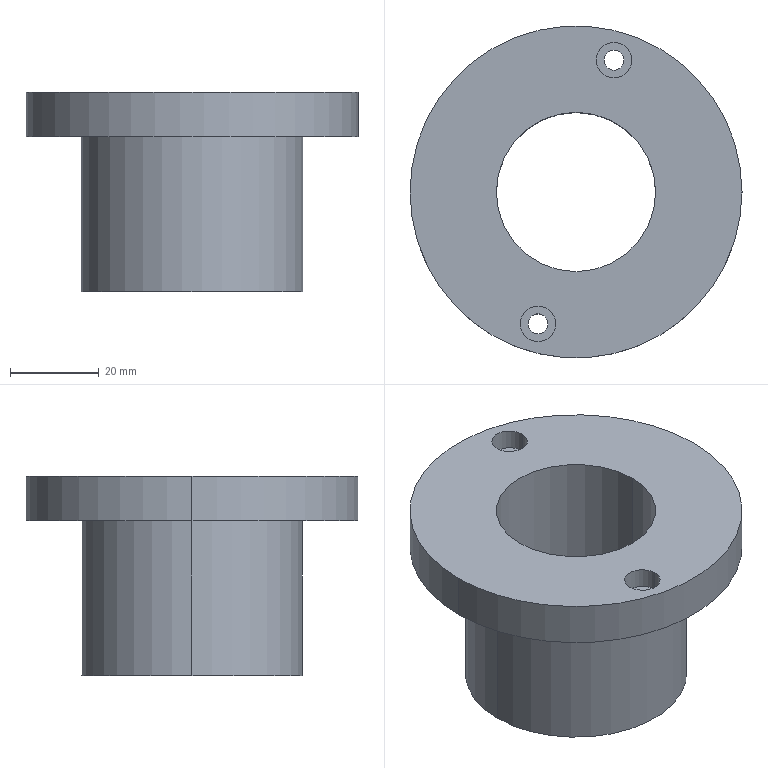Part | SolidWorks | features Extrusion 1, HoleWzd 1, ICE 1 | 1 solid | 19 faces | box 75 x 75 x 45 mm | volume 66462 mm3 | cylinder 14 | plane 5 | commonest cylinder face diameters 4.5 x4 8 x4 36 x2 50 x2 75 x2
STEP:
#1=CARTESIAN_POINT('',(-12.588,-29.787,40.4));
#2=VERTEX_POINT('',#1);
#3=CARTESIAN_POINT('',(-4.588,-29.787,40.4));
#4=VERTEX_POINT('',#3);
#5=CARTESIAN_POINT('',(-8.588,-29.787,40.4));
#6=DIRECTION('',(0.,0.,1.));
#7=DIRECTION('',(1.,0.,0.));
#8=AXIS2_PLACEMENT_3D('',#5,#6,#7);
#9=CIRCLE('',#8,4.);
#10=EDGE_CURVE('',#2,#4,#9,.T.);
#11=ORIENTED_EDGE('',*,*,#10,.F.);
#12=CARTESIAN_POINT('',(-12.588,-29.787,45.));
#13=VERTEX_POINT('',#12);
#14=CARTESIAN_POINT('',(-12.588,-29.787,45.));
#15=DIRECTION('',(0.,0.,1.));
#16=VECTOR('',#15,1000.);
#17=LINE('',#14,#16);
#18=EDGE_CURVE('',#2,#13,#17,.T.);
#19=ORIENTED_EDGE('',*,*,#18,.T.);
#20=CARTESIAN_POINT('',(-4.588,-29.787,45.));
#21=VERTEX_POINT('',#20);
#22=CARTESIAN_POINT('',(-8.588,-29.787,45.));
#23=DIRECTION('',(0.,0.,1.));
#24=DIRECTION('',(1.,0.,0.));
#25=AXIS2_PLACEMENT_3D('',#22,#23,#24);
#26=CIRCLE('',#25,4.);
#27=EDGE_CURVE('',#13,#21,#26,.T.);
#28=ORIENTED_EDGE('',*,*,#27,.T.);
#29=CARTESIAN_POINT('',(-4.588,-29.787,45.));
#30=DIRECTION('',(0.,0.,1.));
#31=VECTOR('',#30,1000.);
#32=LINE('',#29,#31);
#33=EDGE_CURVE('',#4,#21,#32,.T.);
#34=ORIENTED_EDGE('',*,*,#33,.F.);
#35=EDGE_LOOP('',(#11,#19,#28,#34));
#36=FACE_OUTER_BOUND('',#35,.T.);
#37=CARTESIAN_POINT('',(-8.588,-29.787,45.));
#38=DIRECTION('',(0.,0.,1.));
#39=DIRECTION('',(1.,0.,0.));
#40=AXIS2_PLACEMENT_3D('',#37,#38,#39);
#41=CYLINDRICAL_SURFACE('',#40,4.);
#42=ADVANCED_FACE('',(#36),#41,.F.);
#43=CARTESIAN_POINT('',(-10.838,-29.787,35.));
#44=VERTEX_POINT('',#43);
#45=CARTESIAN_POINT('',(-6.338,-29.787,35.));
#46=VERTEX_POINT('',#45);
#47=CARTESIAN_POINT('',(-8.588,-29.787,35.));
#48=DIRECTION('',(0.,0.,1.));
#49=DIRECTION('',(1.,0.,0.));
#50=AXIS2_PLACEMENT_3D('',#47,#48,#49);
#51=CIRCLE('',#50,2.25);
#52=EDGE_CURVE('',#44,#46,#51,.T.);
#53=ORIENTED_EDGE('',*,*,#52,.F.);
#54=CARTESIAN_POINT('',(-10.838,-29.787,40.4));
#55=VERTEX_POINT('',#54);
#56=CARTESIAN_POINT('',(-10.838,-29.787,45.));
#57=DIRECTION('',(0.,0.,1.));
#58=VECTOR('',#57,1000.);
#59=LINE('',#56,#58);
#60=EDGE_CURVE('',#44,#55,#59,.T.);
#61=ORIENTED_EDGE('',*,*,#60,.T.);
#62=CARTESIAN_POINT('',(-6.338,-29.787,40.4));
#63=VERTEX_POINT('',#62);
#64=CARTESIAN_POINT('',(-8.588,-29.787,40.4));
#65=DIRECTION('',(0.,0.,1.));
#66=DIRECTION('',(1.,0.,0.));
#67=AXIS2_PLACEMENT_3D('',#64,#65,#66);
#68=CIRCLE('',#67,2.25);
#69=EDGE_CURVE('',#55,#63,#68,.T.);
#70=ORIENTED_EDGE('',*,*,#69,.T.);
#71=CARTESIAN_POINT('',(-6.338,-29.787,45.));
#72=DIRECTION('',(0.,0.,1.));
#73=VECTOR('',#72,1000.);
#74=LINE('',#71,#73);
#75=EDGE_CURVE('',#46,#63,#74,.T.);
#76=ORIENTED_EDGE('',*,*,#75,.F.);
#77=EDGE_LOOP('',(#53,#61,#70,#76));
#78=FACE_OUTER_BOUND('',#77,.T.);
#79=CARTESIAN_POINT('',(-8.588,-29.787,45.));
#80=DIRECTION('',(0.,0.,1.));
#81=DIRECTION('',(1.,0.,0.));
#82=AXIS2_PLACEMENT_3D('',#79,#80,#81);
#83=CYLINDRICAL_SURFACE('',#82,2.25);
#84=ADVANCED_FACE('',(#78),#83,.F.);
#85=CARTESIAN_POINT('',(4.588,29.787,40.4));
#86=VERTEX_POINT('',#85);
#87=CARTESIAN_POINT('',(12.588,29.787,40.4));
#88=VERTEX_POINT('',#87);
#89=CARTESIAN_POINT('',(8.588,29.787,40.4));
#90=DIRECTION('',(0.,0.,1.));
#91=DIRECTION('',(1.,0.,0.));
#92=AXIS2_PLACEMENT_3D('',#89,#90,#91);
#93=CIRCLE('',#92,4.);
#94=EDGE_CURVE('',#86,#88,#93,.T.);
#95=ORIENTED_EDGE('',*,*,#94,.F.);
#96=CARTESIAN_POINT('',(4.588,29.787,45.));
#97=VERTEX_POINT('',#96);
#98=CARTESIAN_POINT('',(4.588,29.787,45.));
#99=DIRECTION('',(0.,0.,1.));
#100=VECTOR('',#99,1000.);
#101=LINE('',#98,#100);
#102=EDGE_CURVE('',#86,#97,#101,.T.);
#103=ORIENTED_EDGE('',*,*,#102,.T.);
#104=CARTESIAN_POINT('',(12.588,29.787,45.));
#105=VERTEX_POINT('',#104);
#106=CARTESIAN_POINT('',(8.588,29.787,45.));
#107=DIRECTION('',(0.,0.,1.));
#108=DIRECTION('',(1.,0.,0.));
#109=AXIS2_PLACEMENT_3D('',#106,#107,#108);
#110=CIRCLE('',#109,4.);
#111=EDGE_CURVE('',#97,#105,#110,.T.);
#112=ORIENTED_EDGE('',*,*,#111,.T.);
#113=CARTESIAN_POINT('',(12.588,29.787,45.));
#114=DIRECTION('',(0.,0.,1.));
#115=VECTOR('',#114,1000.);
#116=LINE('',#113,#115);
#117=EDGE_CURVE('',#88,#105,#116,.T.);
#118=ORIENTED_EDGE('',*,*,#117,.F.);
#119=EDGE_LOOP('',(#95,#103,#112,#118));
#120=FACE_OUTER_BOUND('',#119,.T.);
#121=CARTESIAN_POINT('',(8.588,29.787,45.));
#122=DIRECTION('',(0.,0.,1.));
#123=DIRECTION('',(1.,0.,0.));
#124=AXIS2_PLACEMENT_3D('',#121,#122,#123);
#125=CYLINDRICAL_SURFACE('',#124,4.);
#126=ADVANCED_FACE('',(#120),#125,.F.);
#127=CARTESIAN_POINT('',(6.338,29.787,35.));
#128=VERTEX_POINT('',#127);
#129=CARTESIAN_POINT('',(10.838,29.787,35.));
#130=VERTEX_POINT('',#129);
#131=CARTESIAN_POINT('',(8.588,29.787,35.));
#132=DIRECTION('',(0.,0.,1.));
#133=DIRECTION('',(1.,0.,0.));
#134=AXIS2_PLACEMENT_3D('',#131,#132,#133);
#135=CIRCLE('',#134,2.25);
#136=EDGE_CURVE('',#128,#130,#135,.T.);
#137=ORIENTED_EDGE('',*,*,#136,.F.);
#138=CARTESIAN_POINT('',(6.338,29.787,40.4));
#139=VERTEX_POINT('',#138);
#140=CARTESIAN_POINT('',(6.338,29.787,45.));
#141=DIRECTION('',(0.,0.,1.));
#142=VECTOR('',#141,1000.);
#143=LINE('',#140,#142);
#144=EDGE_CURVE('',#128,#139,#143,.T.);
#145=ORIENTED_EDGE('',*,*,#144,.T.);
#146=CARTESIAN_POINT('',(10.838,29.787,40.4));
#147=VERTEX_POINT('',#146);
#148=CARTESIAN_POINT('',(8.588,29.787,40.4));
#149=DIRECTION('',(0.,0.,1.));
#150=DIRECTION('',(1.,0.,0.));
#151=AXIS2_PLACEMENT_3D('',#148,#149,#150);
#152=CIRCLE('',#151,2.25);
#153=EDGE_CURVE('',#139,#147,#152,.T.);
#154=ORIENTED_EDGE('',*,*,#153,.T.);
#155=CARTESIAN_POINT('',(10.838,29.787,45.));
#156=DIRECTION('',(0.,0.,1.));
#157=VECTOR('',#156,1000.);
#158=LINE('',#155,#157);
#159=EDGE_CURVE('',#130,#147,#158,.T.);
#160=ORIENTED_EDGE('',*,*,#159,.F.);
#161=EDGE_LOOP('',(#137,#145,#154,#160));
#162=FACE_OUTER_BOUND('',#161,.T.);
#163=CARTESIAN_POINT('',(8.588,29.787,45.));
#164=DIRECTION('',(0.,0.,1.));
#165=DIRECTION('',(1.,0.,0.));
#166=AXIS2_PLACEMENT_3D('',#163,#164,#165);
#167=CYLINDRICAL_SURFACE('',#166,2.25);
#168=ADVANCED_FACE('',(#162),#167,.F.);
#169=CARTESIAN_POINT('',(37.5,0.,45.));
#170=VERTEX_POINT('',#169);
#171=CARTESIAN_POINT('',(-37.5,0.,45.));
#172=VERTEX_POINT('',#171);
#173=CARTESIAN_POINT('',(0.,0.,45.));
#174=DIRECTION('',(0.,0.,1.));
#175=DIRECTION('',(1.,0.,0.));
#176=AXIS2_PLACEMENT_3D('',#173,#174,#175);
#177=CIRCLE('',#176,37.5);
#178=EDGE_CURVE('',#170,#172,#177,.T.);
#179=ORIENTED_EDGE('',*,*,#178,.F.);
#180=CARTESIAN_POINT('',(37.5,0.,35.));
#181=VERTEX_POINT('',#180);
#182=CARTESIAN_POINT('',(37.5,0.,45.));
#183=DIRECTION('',(0.,0.,-1.));
#184=VECTOR('',#183,1000.);
#185=LINE('',#182,#184);
#186=EDGE_CURVE('',#170,#181,#185,.T.);
#187=ORIENTED_EDGE('',*,*,#186,.T.);
#188=CARTESIAN_POINT('',(-37.5,0.,35.));
#189=VERTEX_POINT('',#188);
#190=CARTESIAN_POINT('',(0.,0.,35.));
#191=DIRECTION('',(0.,0.,1.));
#192=DIRECTION('',(1.,0.,0.));
#193=AXIS2_PLACEMENT_3D('',#190,#191,#192);
#194=CIRCLE('',#193,37.5);
#195=EDGE_CURVE('',#181,#189,#194,.T.);
#196=ORIENTED_EDGE('',*,*,#195,.T.);
#197=CARTESIAN_POINT('',(-37.5,0.,45.));
#198=DIRECTION('',(0.,0.,-1.));
#199=VECTOR('',#198,1000.);
#200=LINE('',#197,#199);
#201=EDGE_CURVE('',#172,#189,#200,.T.);
#202=ORIENTED_EDGE('',*,*,#201,.F.);
#203=EDGE_LOOP('',(#179,#187,#196,#202));
#204=FACE_OUTER_BOUND('',#203,.T.);
#205=CARTESIAN_POINT('',(0.,0.,45.));
#206=DIRECTION('',(0.,0.,-1.));
#207=DIRECTION('',(-1.,0.,0.));
#208=AXIS2_PLACEMENT_3D('',#205,#206,#207);
#209=CYLINDRICAL_SURFACE('',#208,37.5);
#210=ADVANCED_FACE('',(#204),#209,.T.);
#211=CARTESIAN_POINT('',(-18.,0.,45.));
#212=VERTEX_POINT('',#211);
#213=CARTESIAN_POINT('',(18.,0.,45.));
#214=VERTEX_POINT('',#213);
#215=CARTESIAN_POINT('',(0.,0.,45.));
#216=DIRECTION('',(0.,0.,1.));
#217=DIRECTION('',(1.,0.,0.));
#218=AXIS2_PLACEMENT_3D('',#215,#216,#217);
#219=CIRCLE('',#218,18.);
#220=EDGE_CURVE('',#212,#214,#219,.T.);
#221=ORIENTED_EDGE('',*,*,#220,.T.);
#222=CARTESIAN_POINT('',(18.,0.,0.));
#223=VERTEX_POINT('',#222);
#224=CARTESIAN_POINT('',(18.,0.,35.));
#225=DIRECTION('',(0.,0.,-1.));
#226=VECTOR('',#225,1000.);
#227=LINE('',#224,#226);
#228=EDGE_CURVE('',#214,#223,#227,.T.);
#229=ORIENTED_EDGE('',*,*,#228,.T.);
#230=CARTESIAN_POINT('',(-18.,0.,0.));
#231=VERTEX_POINT('',#230);
#232=CARTESIAN_POINT('',(0.,0.,0.));
#233=DIRECTION('',(0.,0.,1.));
#234=DIRECTION('',(1.,0.,0.));
#235=AXIS2_PLACEMENT_3D('',#232,#233,#234);
#236=CIRCLE('',#235,18.);
#237=EDGE_CURVE('',#231,#223,#236,.T.);
#238=ORIENTED_EDGE('',*,*,#237,.F.);
#239=CARTESIAN_POINT('',(-18.,0.,35.));
#240=DIRECTION('',(0.,0.,-1.));
#241=VECTOR('',#240,1000.);
#242=LINE('',#239,#241);
#243=EDGE_CURVE('',#212,#231,#242,.T.);
#244=ORIENTED_EDGE('',*,*,#243,.F.);
#245=EDGE_LOOP('',(#221,#229,#238,#244));
#246=FACE_OUTER_BOUND('',#245,.T.);
#247=CARTESIAN_POINT('',(0.,0.,35.));
#248=DIRECTION('',(0.,0.,-1.));
#249=DIRECTION('',(-1.,0.,0.));
#250=AXIS2_PLACEMENT_3D('',#247,#248,#249);
#251=CYLINDRICAL_SURFACE('',#250,18.);
#252=ADVANCED_FACE('',(#246),#251,.F.);
#253=CARTESIAN_POINT('',(25.,0.,35.));
#254=VERTEX_POINT('',#253);
#255=CARTESIAN_POINT('',(-25.,0.,35.));
#256=VERTEX_POINT('',#255);
#257=CARTESIAN_POINT('',(0.,0.,35.));
#258=DIRECTION('',(0.,0.,1.));
#259=DIRECTION('',(1.,0.,0.));
#260=AXIS2_PLACEMENT_3D('',#257,#258,#259);
#261=CIRCLE('',#260,25.);
#262=EDGE_CURVE('',#254,#256,#261,.T.);
#263=ORIENTED_EDGE('',*,*,#262,.F.);
#264=CARTESIAN_POINT('',(25.,0.,0.));
#265=VERTEX_POINT('',#264);
#266=CARTESIAN_POINT('',(25.,0.,35.));
#267=DIRECTION('',(0.,0.,-1.));
#268=VECTOR('',#267,1000.);
#269=LINE('',#266,#268);
#270=EDGE_CURVE('',#254,#265,#269,.T.);
#271=ORIENTED_EDGE('',*,*,#270,.T.);
#272=CARTESIAN_POINT('',(-25.,0.,0.));
#273=VERTEX_POINT('',#272);
#274=CARTESIAN_POINT('',(0.,0.,0.));
#275=DIRECTION('',(0.,0.,1.));
#276=DIRECTION('',(1.,0.,0.));
#277=AXIS2_PLACEMENT_3D('',#274,#275,#276);
#278=CIRCLE('',#277,25.);
#279=EDGE_CURVE('',#265,#273,#278,.T.);
#280=ORIENTED_EDGE('',*,*,#279,.T.);
#281=CARTESIAN_POINT('',(-25.,0.,35.));
#282=DIRECTION('',(0.,0.,-1.));
#283=VECTOR('',#282,1000.);
#284=LINE('',#281,#283);
#285=EDGE_CURVE('',#256,#273,#284,.T.);
#286=ORIENTED_EDGE('',*,*,#285,.F.);
#287=EDGE_LOOP('',(#263,#271,#280,#286));
#288=FACE_OUTER_BOUND('',#287,.T.);
#289=CARTESIAN_POINT('',(0.,0.,35.));
#290=DIRECTION('',(0.,0.,-1.));
#291=DIRECTION('',(-1.,0.,0.));
#292=AXIS2_PLACEMENT_3D('',#289,#290,#291);
#293=CYLINDRICAL_SURFACE('',#292,25.);
#294=ADVANCED_FACE('',(#288),#293,.T.);
#295=CARTESIAN_POINT('',(0.,0.,0.));
#296=DIRECTION('',(0.,0.,1.));
#297=DIRECTION('',(1.,0.,0.));
#298=AXIS2_PLACEMENT_3D('',#295,#296,#297);
#299=CIRCLE('',#298,25.);
#300=EDGE_CURVE('',#273,#265,#299,.T.);
#301=ORIENTED_EDGE('',*,*,#300,.F.);
#302=ORIENTED_EDGE('',*,*,#279,.F.);
#303=EDGE_LOOP('',(#301,#302));
#304=FACE_OUTER_BOUND('',#303,.T.);
#305=ORIENTED_EDGE('',*,*,#237,.T.);
#306=CARTESIAN_POINT('',(0.,0.,0.));
#307=DIRECTION('',(0.,0.,1.));
#308=DIRECTION('',(1.,0.,0.));
#309=AXIS2_PLACEMENT_3D('',#306,#307,#308);
#310=CIRCLE('',#309,18.);
#311=EDGE_CURVE('',#223,#231,#310,.T.);
#312=ORIENTED_EDGE('',*,*,#311,.T.);
#313=EDGE_LOOP('',(#305,#312));
#314=FACE_BOUND('',#313,.T.);
#315=CARTESIAN_POINT('',(0.,0.,0.));
#316=DIRECTION('',(0.,0.,1.));
#317=DIRECTION('',(1.,0.,0.));
#318=AXIS2_PLACEMENT_3D('',#315,#316,#317);
#319=PLANE('',#318);
#320=ADVANCED_FACE('',(#304,#314),#319,.F.);
#321=ORIENTED_EDGE('',*,*,#270,.F.);
#322=CARTESIAN_POINT('',(0.,0.,35.));
#323=DIRECTION('',(0.,0.,1.));
#324=DIRECTION('',(1.,0.,0.));
#325=AXIS2_PLACEMENT_3D('',#322,#323,#324);
#326=CIRCLE('',#325,25.);
#327=EDGE_CURVE('',#256,#254,#326,.T.);
#328=ORIENTED_EDGE('',*,*,#327,.F.);
#329=ORIENTED_EDGE('',*,*,#285,.T.);
#330=ORIENTED_EDGE('',*,*,#300,.T.);
#331=EDGE_LOOP('',(#321,#328,#329,#330));
#332=FACE_OUTER_BOUND('',#331,.T.);
#333=CARTESIAN_POINT('',(0.,0.,35.));
#334=DIRECTION('',(0.,0.,-1.));
#335=DIRECTION('',(-1.,0.,0.));
#336=AXIS2_PLACEMENT_3D('',#333,#334,#335);
#337=CYLINDRICAL_SURFACE('',#336,25.);
#338=ADVANCED_FACE('',(#332),#337,.T.);
#339=ORIENTED_EDGE('',*,*,#228,.F.);
#340=CARTESIAN_POINT('',(0.,0.,45.));
#341=DIRECTION('',(0.,0.,1.));
#342=DIRECTION('',(1.,0.,0.));
#343=AXIS2_PLACEMENT_3D('',#340,#341,#342);
#344=CIRCLE('',#343,18.);
#345=EDGE_CURVE('',#214,#212,#344,.T.);
#346=ORIENTED_EDGE('',*,*,#345,.T.);
#347=ORIENTED_EDGE('',*,*,#243,.T.);
#348=ORIENTED_EDGE('',*,*,#311,.F.);
#349=EDGE_LOOP('',(#339,#346,#347,#348));
#350=FACE_OUTER_BOUND('',#349,.T.);
#351=CARTESIAN_POINT('',(0.,0.,35.));
#352=DIRECTION('',(0.,0.,-1.));
#353=DIRECTION('',(-1.,0.,0.));
#354=AXIS2_PLACEMENT_3D('',#351,#352,#353);
#355=CYLINDRICAL_SURFACE('',#354,18.);
#356=ADVANCED_FACE('',(#350),#355,.F.);
#357=CARTESIAN_POINT('',(-8.588,-29.787,45.));
#358=DIRECTION('',(0.,0.,1.));
#359=DIRECTION('',(1.,0.,0.));
#360=AXIS2_PLACEMENT_3D('',#357,#358,#359);
#361=CIRCLE('',#360,4.);
#362=EDGE_CURVE('',#21,#13,#361,.T.);
#363=ORIENTED_EDGE('',*,*,#362,.F.);
#364=ORIENTED_EDGE('',*,*,#27,.F.);
#365=EDGE_LOOP('',(#363,#364));
#366=FACE_BOUND('',#365,.T.);
#367=CARTESIAN_POINT('',(8.588,29.787,45.));
#368=DIRECTION('',(0.,0.,1.));
#369=DIRECTION('',(1.,0.,0.));
#370=AXIS2_PLACEMENT_3D('',#367,#368,#369);
#371=CIRCLE('',#370,4.);
#372=EDGE_CURVE('',#105,#97,#371,.T.);
#373=ORIENTED_EDGE('',*,*,#372,.F.);
#374=ORIENTED_EDGE('',*,*,#111,.F.);
#375=EDGE_LOOP('',(#373,#374));
#376=FACE_BOUND('',#375,.T.);
#377=CARTESIAN_POINT('',(0.,0.,45.));
#378=DIRECTION('',(0.,0.,1.));
#379=DIRECTION('',(1.,0.,0.));
#380=AXIS2_PLACEMENT_3D('',#377,#378,#379);
#381=CIRCLE('',#380,37.5);
#382=EDGE_CURVE('',#172,#170,#381,.T.);
#383=ORIENTED_EDGE('',*,*,#382,.T.);
#384=ORIENTED_EDGE('',*,*,#178,.T.);
#385=EDGE_LOOP('',(#383,#384));
#386=FACE_OUTER_BOUND('',#385,.T.);
#387=ORIENTED_EDGE('',*,*,#220,.F.);
#388=ORIENTED_EDGE('',*,*,#345,.F.);
#389=EDGE_LOOP('',(#387,#388));
#390=FACE_BOUND('',#389,.T.);
#391=CARTESIAN_POINT('',(0.,0.,45.));
#392=DIRECTION('',(0.,0.,1.));
#393=DIRECTION('',(1.,0.,0.));
#394=AXIS2_PLACEMENT_3D('',#391,#392,#393);
#395=PLANE('',#394);
#396=ADVANCED_FACE('',(#366,#376,#386,#390),#395,.T.);
#397=CARTESIAN_POINT('',(-8.588,-29.787,35.));
#398=DIRECTION('',(0.,0.,1.));
#399=DIRECTION('',(1.,0.,0.));
#400=AXIS2_PLACEMENT_3D('',#397,#398,#399);
#401=CIRCLE('',#400,2.25);
#402=EDGE_CURVE('',#46,#44,#401,.T.);
#403=ORIENTED_EDGE('',*,*,#402,.T.);
#404=ORIENTED_EDGE('',*,*,#52,.T.);
#405=EDGE_LOOP('',(#403,#404));
#406=FACE_BOUND('',#405,.T.);
#407=CARTESIAN_POINT('',(8.588,29.787,35.));
#408=DIRECTION('',(0.,0.,1.));
#409=DIRECTION('',(1.,0.,0.));
#410=AXIS2_PLACEMENT_3D('',#407,#408,#409);
#411=CIRCLE('',#410,2.25);
#412=EDGE_CURVE('',#130,#128,#411,.T.);
#413=ORIENTED_EDGE('',*,*,#412,.T.);
#414=ORIENTED_EDGE('',*,*,#136,.T.);
#415=EDGE_LOOP('',(#413,#414));
#416=FACE_BOUND('',#415,.T.);
#417=ORIENTED_EDGE('',*,*,#327,.T.);
#418=ORIENTED_EDGE('',*,*,#262,.T.);
#419=EDGE_LOOP('',(#417,#418));
#420=FACE_BOUND('',#419,.T.);
#421=CARTESIAN_POINT('',(0.,0.,35.));
#422=DIRECTION('',(0.,0.,1.));
#423=DIRECTION('',(1.,0.,0.));
#424=AXIS2_PLACEMENT_3D('',#421,#422,#423);
#425=CIRCLE('',#424,37.5);
#426=EDGE_CURVE('',#189,#181,#425,.T.);
#427=ORIENTED_EDGE('',*,*,#426,.F.);
#428=ORIENTED_EDGE('',*,*,#195,.F.);
#429=EDGE_LOOP('',(#427,#428));
#430=FACE_OUTER_BOUND('',#429,.T.);
#431=CARTESIAN_POINT('',(0.,0.,35.));
#432=DIRECTION('',(0.,0.,1.));
#433=DIRECTION('',(1.,0.,0.));
#434=AXIS2_PLACEMENT_3D('',#431,#432,#433);
#435=PLANE('',#434);
#436=ADVANCED_FACE('',(#406,#416,#420,#430),#435,.F.);
#437=ORIENTED_EDGE('',*,*,#186,.F.);
#438=ORIENTED_EDGE('',*,*,#382,.F.);
#439=ORIENTED_EDGE('',*,*,#201,.T.);
#440=ORIENTED_EDGE('',*,*,#426,.T.);
#441=EDGE_LOOP('',(#437,#438,#439,#440));
#442=FACE_OUTER_BOUND('',#441,.T.);
#443=CARTESIAN_POINT('',(0.,0.,45.));
#444=DIRECTION('',(0.,0.,-1.));
#445=DIRECTION('',(-1.,0.,0.));
#446=AXIS2_PLACEMENT_3D('',#443,#444,#445);
#447=CYLINDRICAL_SURFACE('',#446,37.5);
#448=ADVANCED_FACE('',(#442),#447,.T.);
#449=ORIENTED_EDGE('',*,*,#144,.F.);
#450=ORIENTED_EDGE('',*,*,#412,.F.);
#451=ORIENTED_EDGE('',*,*,#159,.T.);
#452=CARTESIAN_POINT('',(8.588,29.787,40.4));
#453=DIRECTION('',(0.,0.,1.));
#454=DIRECTION('',(1.,0.,0.));
#455=AXIS2_PLACEMENT_3D('',#452,#453,#454);
#456=CIRCLE('',#455,2.25);
#457=EDGE_CURVE('',#147,#139,#456,.T.);
#458=ORIENTED_EDGE('',*,*,#457,.T.);
#459=EDGE_LOOP('',(#449,#450,#451,#458));
#460=FACE_OUTER_BOUND('',#459,.T.);
#461=CARTESIAN_POINT('',(8.588,29.787,45.));
#462=DIRECTION('',(0.,0.,1.));
#463=DIRECTION('',(1.,0.,0.));
#464=AXIS2_PLACEMENT_3D('',#461,#462,#463);
#465=CYLINDRICAL_SURFACE('',#464,2.25);
#466=ADVANCED_FACE('',(#460),#465,.F.);
#467=ORIENTED_EDGE('',*,*,#457,.F.);
#468=ORIENTED_EDGE('',*,*,#153,.F.);
#469=EDGE_LOOP('',(#467,#468));
#470=FACE_BOUND('',#469,.T.);
#471=CARTESIAN_POINT('',(8.588,29.787,40.4));
#472=DIRECTION('',(0.,0.,1.));
#473=DIRECTION('',(1.,0.,0.));
#474=AXIS2_PLACEMENT_3D('',#471,#472,#473);
#475=CIRCLE('',#474,4.);
#476=EDGE_CURVE('',#88,#86,#475,.T.);
#477=ORIENTED_EDGE('',*,*,#476,.T.);
#478=ORIENTED_EDGE('',*,*,#94,.T.);
#479=EDGE_LOOP('',(#477,#478));
#480=FACE_OUTER_BOUND('',#479,.T.);
#481=CARTESIAN_POINT('',(10.838,29.787,40.4));
#482=DIRECTION('',(0.,0.,-1.));
#483=DIRECTION('',(-1.,0.,0.));
#484=AXIS2_PLACEMENT_3D('',#481,#482,#483);
#485=PLANE('',#484);
#486=ADVANCED_FACE('',(#470,#480),#485,.F.);
#487=ORIENTED_EDGE('',*,*,#102,.F.);
#488=ORIENTED_EDGE('',*,*,#476,.F.);
#489=ORIENTED_EDGE('',*,*,#117,.T.);
#490=ORIENTED_EDGE('',*,*,#372,.T.);
#491=EDGE_LOOP('',(#487,#488,#489,#490));
#492=FACE_OUTER_BOUND('',#491,.T.);
#493=CARTESIAN_POINT('',(8.588,29.787,45.));
#494=DIRECTION('',(0.,0.,1.));
#495=DIRECTION('',(1.,0.,0.));
#496=AXIS2_PLACEMENT_3D('',#493,#494,#495);
#497=CYLINDRICAL_SURFACE('',#496,4.);
#498=ADVANCED_FACE('',(#492),#497,.F.);
#499=ORIENTED_EDGE('',*,*,#60,.F.);
#500=ORIENTED_EDGE('',*,*,#402,.F.);
#501=ORIENTED_EDGE('',*,*,#75,.T.);
#502=CARTESIAN_POINT('',(-8.588,-29.787,40.4));
#503=DIRECTION('',(0.,0.,1.));
#504=DIRECTION('',(1.,0.,0.));
#505=AXIS2_PLACEMENT_3D('',#502,#503,#504);
#506=CIRCLE('',#505,2.25);
#507=EDGE_CURVE('',#63,#55,#506,.T.);
#508=ORIENTED_EDGE('',*,*,#507,.T.);
#509=EDGE_LOOP('',(#499,#500,#501,#508));
#510=FACE_OUTER_BOUND('',#509,.T.);
#511=CARTESIAN_POINT('',(-8.588,-29.787,45.));
#512=DIRECTION('',(0.,0.,1.));
#513=DIRECTION('',(1.,0.,0.));
#514=AXIS2_PLACEMENT_3D('',#511,#512,#513);
#515=CYLINDRICAL_SURFACE('',#514,2.25);
#516=ADVANCED_FACE('',(#510),#515,.F.);
#517=ORIENTED_EDGE('',*,*,#507,.F.);
#518=ORIENTED_EDGE('',*,*,#69,.F.);
#519=EDGE_LOOP('',(#517,#518));
#520=FACE_BOUND('',#519,.T.);
#521=CARTESIAN_POINT('',(-8.588,-29.787,40.4));
#522=DIRECTION('',(0.,0.,1.));
#523=DIRECTION('',(1.,0.,0.));
#524=AXIS2_PLACEMENT_3D('',#521,#522,#523);
#525=CIRCLE('',#524,4.);
#526=EDGE_CURVE('',#4,#2,#525,.T.);
#527=ORIENTED_EDGE('',*,*,#526,.T.);
#528=ORIENTED_EDGE('',*,*,#10,.T.);
#529=EDGE_LOOP('',(#527,#528));
#530=FACE_OUTER_BOUND('',#529,.T.);
#531=CARTESIAN_POINT('',(-6.338,-29.787,40.4));
#532=DIRECTION('',(0.,0.,-1.));
#533=DIRECTION('',(-1.,0.,0.));
#534=AXIS2_PLACEMENT_3D('',#531,#532,#533);
#535=PLANE('',#534);
#536=ADVANCED_FACE('',(#520,#530),#535,.F.);
#537=ORIENTED_EDGE('',*,*,#18,.F.);
#538=ORIENTED_EDGE('',*,*,#526,.F.);
#539=ORIENTED_EDGE('',*,*,#33,.T.);
#540=ORIENTED_EDGE('',*,*,#362,.T.);
#541=EDGE_LOOP('',(#537,#538,#539,#540));
#542=FACE_OUTER_BOUND('',#541,.T.);
#543=CARTESIAN_POINT('',(-8.588,-29.787,45.));
#544=DIRECTION('',(0.,0.,1.));
#545=DIRECTION('',(1.,0.,0.));
#546=AXIS2_PLACEMENT_3D('',#543,#544,#545);
#547=CYLINDRICAL_SURFACE('',#546,4.);
#548=ADVANCED_FACE('',(#542),#547,.F.);
#549=CLOSED_SHELL('',(#42,#84,#126,#168,#210,#252,#294,#320,#338,#356,#396,#436,#448,#466,#486,#498,#516,#536,#548));
#550=MANIFOLD_SOLID_BREP('',#549);
#551=CARTESIAN_POINT('',(0.,0.,0.));
#552=DIRECTION('',(0.,0.,1.));
#553=DIRECTION('',(1.,0.,0.));
#554=AXIS2_PLACEMENT_3D('',#551,#552,#553);
#555=(LENGTH_UNIT()NAMED_UNIT(*)SI_UNIT(.MILLI.,.METRE.));
#556=UNCERTAINTY_MEASURE_WITH_UNIT(LENGTH_MEASURE(0.00001),#555,'','');
#557=(NAMED_UNIT(*)PLANE_ANGLE_UNIT()SI_UNIT($,.RADIAN.));
#558=(NAMED_UNIT(*)SI_UNIT($,.STERADIAN.)SOLID_ANGLE_UNIT());
#559=(GEOMETRIC_REPRESENTATION_CONTEXT(3)GLOBAL_UNCERTAINTY_ASSIGNED_CONTEXT((#556))GLOBAL_UNIT_ASSIGNED_CONTEXT((#555,#557,#558))REPRESENTATION_CONTEXT('',''));
#560=ADVANCED_BREP_SHAPE_REPRESENTATION('',(#550,#554),#559);